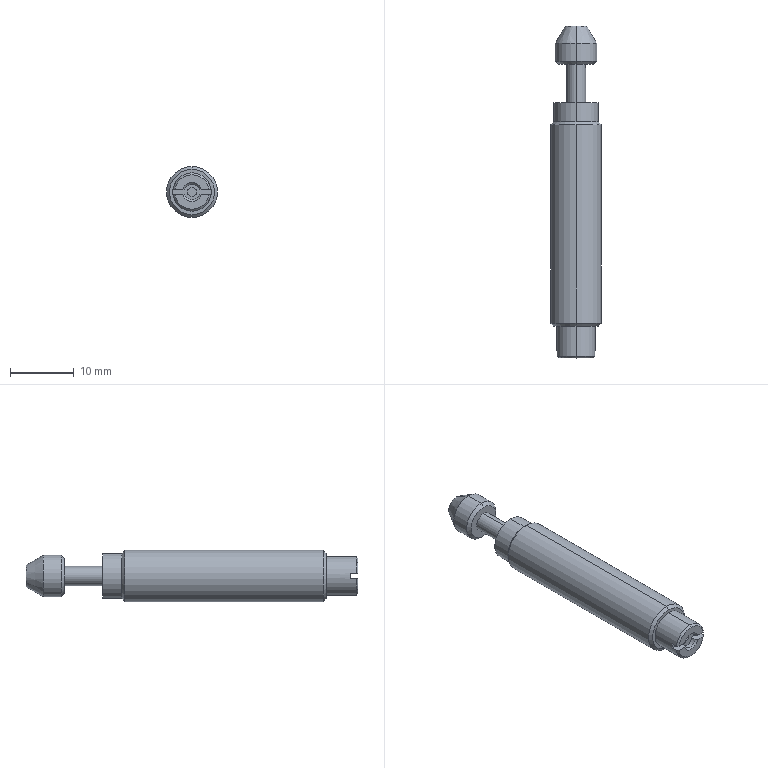Part | SolidWorks | features BaseBody 1 | 1 solid | 46 faces | box 8 x 52 x 8 mm | volume 2052 mm3 | plane 19 | cone 15 | cylinder 12 | commonest cylinder face diameters 2.459 x2 3 x2 6 x2 6.5 x2 7 x2 8 x2
STEP:
#1=CARTESIAN_POINT('',(0.,5.46,4.));
#2=VERTEX_POINT('',#1);
#3=CARTESIAN_POINT('',(0.,5.46,-4.));
#4=VERTEX_POINT('',#3);
#5=CARTESIAN_POINT('',(0.,5.46,0.));
#6=DIRECTION('',(0.,1.,0.));
#7=DIRECTION('',(0.,0.,1.));
#8=AXIS2_PLACEMENT_3D('',#5,#6,#7);
#9=CIRCLE('',#8,4.);
#10=EDGE_CURVE('',#2,#4,#9,.T.);
#11=ORIENTED_EDGE('',*,*,#10,.T.);
#12=CARTESIAN_POINT('',(0.,36.54,-4.));
#13=VERTEX_POINT('',#12);
#14=CARTESIAN_POINT('',(0.,0.,-4.));
#15=DIRECTION('',(0.,1.,0.));
#16=VECTOR('',#15,1000.);
#17=LINE('',#14,#16);
#18=EDGE_CURVE('',#4,#13,#17,.T.);
#19=ORIENTED_EDGE('',*,*,#18,.T.);
#20=CARTESIAN_POINT('',(0.,36.54,4.));
#21=VERTEX_POINT('',#20);
#22=CARTESIAN_POINT('',(0.,36.54,0.));
#23=DIRECTION('',(0.,-1.,0.));
#24=DIRECTION('',(0.,0.,1.));
#25=AXIS2_PLACEMENT_3D('',#22,#23,#24);
#26=CIRCLE('',#25,4.);
#27=EDGE_CURVE('',#13,#21,#26,.T.);
#28=ORIENTED_EDGE('',*,*,#27,.T.);
#29=CARTESIAN_POINT('',(0.,0.,4.));
#30=DIRECTION('',(0.,1.,0.));
#31=VECTOR('',#30,1000.);
#32=LINE('',#29,#31);
#33=EDGE_CURVE('',#2,#21,#32,.T.);
#34=ORIENTED_EDGE('',*,*,#33,.F.);
#35=EDGE_LOOP('',(#11,#19,#28,#34));
#36=FACE_OUTER_BOUND('',#35,.T.);
#37=CARTESIAN_POINT('',(0.,0.,0.));
#38=DIRECTION('',(0.,1.,0.));
#39=DIRECTION('',(0.,0.,1.));
#40=AXIS2_PLACEMENT_3D('',#37,#38,#39);
#41=CYLINDRICAL_SURFACE('',#40,4.);
#42=ADVANCED_FACE('',(#36),#41,.T.);
#43=CARTESIAN_POINT('',(0.,37.,-3.54));
#44=VERTEX_POINT('',#43);
#45=CARTESIAN_POINT('',(0.,37.,3.54));
#46=VERTEX_POINT('',#45);
#47=CARTESIAN_POINT('',(0.,37.,0.));
#48=DIRECTION('',(0.,-1.,0.));
#49=DIRECTION('',(0.,0.,-1.));
#50=AXIS2_PLACEMENT_3D('',#47,#48,#49);
#51=CIRCLE('',#50,3.54);
#52=EDGE_CURVE('',#44,#46,#51,.T.);
#53=ORIENTED_EDGE('',*,*,#52,.T.);
#54=CARTESIAN_POINT('',(0.,36.54,4.));
#55=DIRECTION('',(0.,-0.7071,0.7071));
#56=VECTOR('',#55,1000.);
#57=LINE('',#54,#56);
#58=EDGE_CURVE('',#46,#21,#57,.T.);
#59=ORIENTED_EDGE('',*,*,#58,.T.);
#60=ORIENTED_EDGE('',*,*,#27,.F.);
#61=CARTESIAN_POINT('',(0.,36.54,-4.));
#62=DIRECTION('',(0.,-0.7071,-0.7071));
#63=VECTOR('',#62,1000.);
#64=LINE('',#61,#63);
#65=EDGE_CURVE('',#44,#13,#64,.T.);
#66=ORIENTED_EDGE('',*,*,#65,.F.);
#67=EDGE_LOOP('',(#53,#59,#60,#66));
#68=FACE_OUTER_BOUND('',#67,.T.);
#69=CARTESIAN_POINT('',(0.,36.54,0.));
#70=DIRECTION('',(0.,-1.,0.));
#71=DIRECTION('',(0.,0.,-1.));
#72=AXIS2_PLACEMENT_3D('',#69,#70,#71);
#73=CONICAL_SURFACE('',#72,4.,0.7854);
#74=ADVANCED_FACE('',(#68),#73,.T.);
#75=CARTESIAN_POINT('',(0.,5.,3.54));
#76=VERTEX_POINT('',#75);
#77=CARTESIAN_POINT('',(0.,5.,-3.54));
#78=VERTEX_POINT('',#77);
#79=CARTESIAN_POINT('',(0.,5.,0.));
#80=DIRECTION('',(0.,1.,0.));
#81=DIRECTION('',(0.,0.,1.));
#82=AXIS2_PLACEMENT_3D('',#79,#80,#81);
#83=CIRCLE('',#82,3.54);
#84=EDGE_CURVE('',#76,#78,#83,.T.);
#85=ORIENTED_EDGE('',*,*,#84,.T.);
#86=CARTESIAN_POINT('',(0.,5.46,-4.));
#87=DIRECTION('',(0.,0.7071,-0.7071));
#88=VECTOR('',#87,1000.);
#89=LINE('',#86,#88);
#90=EDGE_CURVE('',#78,#4,#89,.T.);
#91=ORIENTED_EDGE('',*,*,#90,.T.);
#92=ORIENTED_EDGE('',*,*,#10,.F.);
#93=CARTESIAN_POINT('',(0.,5.46,4.));
#94=DIRECTION('',(0.,0.7071,0.7071));
#95=VECTOR('',#94,1000.);
#96=LINE('',#93,#95);
#97=EDGE_CURVE('',#76,#2,#96,.T.);
#98=ORIENTED_EDGE('',*,*,#97,.F.);
#99=EDGE_LOOP('',(#85,#91,#92,#98));
#100=FACE_OUTER_BOUND('',#99,.T.);
#101=CARTESIAN_POINT('',(0.,5.46,0.));
#102=DIRECTION('',(0.,1.,0.));
#103=DIRECTION('',(0.,0.,1.));
#104=AXIS2_PLACEMENT_3D('',#101,#102,#103);
#105=CONICAL_SURFACE('',#104,4.,0.7854);
#106=ADVANCED_FACE('',(#100),#105,.T.);
#107=CARTESIAN_POINT('',(0.,37.,3.5));
#108=VERTEX_POINT('',#107);
#109=CARTESIAN_POINT('',(0.,37.,-3.5));
#110=VERTEX_POINT('',#109);
#111=CARTESIAN_POINT('',(0.,37.,0.));
#112=DIRECTION('',(0.,1.,0.));
#113=DIRECTION('',(0.,0.,1.));
#114=AXIS2_PLACEMENT_3D('',#111,#112,#113);
#115=CIRCLE('',#114,3.5);
#116=EDGE_CURVE('',#108,#110,#115,.T.);
#117=ORIENTED_EDGE('',*,*,#116,.T.);
#118=CARTESIAN_POINT('',(0.,40.,-3.5));
#119=VERTEX_POINT('',#118);
#120=CARTESIAN_POINT('',(0.,0.,-3.5));
#121=DIRECTION('',(0.,1.,0.));
#122=VECTOR('',#121,1000.);
#123=LINE('',#120,#122);
#124=EDGE_CURVE('',#110,#119,#123,.T.);
#125=ORIENTED_EDGE('',*,*,#124,.T.);
#126=CARTESIAN_POINT('',(0.,40.,3.5));
#127=VERTEX_POINT('',#126);
#128=CARTESIAN_POINT('',(0.,40.,0.));
#129=DIRECTION('',(0.,-1.,0.));
#130=DIRECTION('',(0.,0.,1.));
#131=AXIS2_PLACEMENT_3D('',#128,#129,#130);
#132=CIRCLE('',#131,3.5);
#133=EDGE_CURVE('',#119,#127,#132,.T.);
#134=ORIENTED_EDGE('',*,*,#133,.T.);
#135=CARTESIAN_POINT('',(0.,0.,3.5));
#136=DIRECTION('',(0.,1.,0.));
#137=VECTOR('',#136,1000.);
#138=LINE('',#135,#137);
#139=EDGE_CURVE('',#108,#127,#138,.T.);
#140=ORIENTED_EDGE('',*,*,#139,.F.);
#141=EDGE_LOOP('',(#117,#125,#134,#140));
#142=FACE_OUTER_BOUND('',#141,.T.);
#143=CARTESIAN_POINT('',(0.,0.,0.));
#144=DIRECTION('',(0.,1.,0.));
#145=DIRECTION('',(0.,0.,1.));
#146=AXIS2_PLACEMENT_3D('',#143,#144,#145);
#147=CYLINDRICAL_SURFACE('',#146,3.5);
#148=ADVANCED_FACE('',(#142),#147,.T.);
#149=CARTESIAN_POINT('',(2.973,0.3,-0.4));
#150=VERTEX_POINT('',#149);
#151=CARTESIAN_POINT('',(0.,0.3,-3.));
#152=VERTEX_POINT('',#151);
#153=CARTESIAN_POINT('',(0.,0.3,0.));
#154=DIRECTION('',(0.,1.,0.));
#155=DIRECTION('',(0.,0.,1.));
#156=AXIS2_PLACEMENT_3D('',#153,#154,#155);
#157=CIRCLE('',#156,3.);
#158=EDGE_CURVE('',#150,#152,#157,.T.);
#159=ORIENTED_EDGE('',*,*,#158,.T.);
#160=CARTESIAN_POINT('',(0.,5.,-3.));
#161=VERTEX_POINT('',#160);
#162=CARTESIAN_POINT('',(0.,0.,-3.));
#163=DIRECTION('',(0.,1.,0.));
#164=VECTOR('',#163,1000.);
#165=LINE('',#162,#164);
#166=EDGE_CURVE('',#152,#161,#165,.T.);
#167=ORIENTED_EDGE('',*,*,#166,.T.);
#168=CARTESIAN_POINT('',(0.,5.,3.));
#169=VERTEX_POINT('',#168);
#170=CARTESIAN_POINT('',(0.,5.,0.));
#171=DIRECTION('',(0.,-1.,0.));
#172=DIRECTION('',(0.,0.,1.));
#173=AXIS2_PLACEMENT_3D('',#170,#171,#172);
#174=CIRCLE('',#173,3.);
#175=EDGE_CURVE('',#161,#169,#174,.T.);
#176=ORIENTED_EDGE('',*,*,#175,.T.);
#177=CARTESIAN_POINT('',(0.,0.3,3.));
#178=VERTEX_POINT('',#177);
#179=CARTESIAN_POINT('',(0.,0.,3.));
#180=DIRECTION('',(0.,1.,0.));
#181=VECTOR('',#180,1000.);
#182=LINE('',#179,#181);
#183=EDGE_CURVE('',#178,#169,#182,.T.);
#184=ORIENTED_EDGE('',*,*,#183,.F.);
#185=CARTESIAN_POINT('',(2.973,0.3,0.4));
#186=VERTEX_POINT('',#185);
#187=CARTESIAN_POINT('',(0.,0.3,0.));
#188=DIRECTION('',(0.,1.,0.));
#189=DIRECTION('',(0.,0.,1.));
#190=AXIS2_PLACEMENT_3D('',#187,#188,#189);
#191=CIRCLE('',#190,3.);
#192=EDGE_CURVE('',#178,#186,#191,.T.);
#193=ORIENTED_EDGE('',*,*,#192,.T.);
#194=CARTESIAN_POINT('',(2.973,1.2,0.4));
#195=VERTEX_POINT('',#194);
#196=CARTESIAN_POINT('',(2.973,0.,0.4));
#197=DIRECTION('',(0.,1.,0.));
#198=VECTOR('',#197,1000.);
#199=LINE('',#196,#198);
#200=EDGE_CURVE('',#186,#195,#199,.T.);
#201=ORIENTED_EDGE('',*,*,#200,.T.);
#202=CARTESIAN_POINT('',(2.973,1.2,-0.4));
#203=VERTEX_POINT('',#202);
#204=CARTESIAN_POINT('',(0.,1.2,0.));
#205=DIRECTION('',(0.,-1.,0.));
#206=DIRECTION('',(0.,0.,1.));
#207=AXIS2_PLACEMENT_3D('',#204,#205,#206);
#208=CIRCLE('',#207,3.);
#209=EDGE_CURVE('',#203,#195,#208,.T.);
#210=ORIENTED_EDGE('',*,*,#209,.F.);
#211=CARTESIAN_POINT('',(2.973,0.,-0.4));
#212=DIRECTION('',(0.,-1.,0.));
#213=VECTOR('',#212,1000.);
#214=LINE('',#211,#213);
#215=EDGE_CURVE('',#203,#150,#214,.T.);
#216=ORIENTED_EDGE('',*,*,#215,.T.);
#217=EDGE_LOOP('',(#159,#167,#176,#184,#193,#201,#210,#216));
#218=FACE_OUTER_BOUND('',#217,.T.);
#219=CARTESIAN_POINT('',(0.,0.,0.));
#220=DIRECTION('',(0.,1.,0.));
#221=DIRECTION('',(0.,0.,1.));
#222=AXIS2_PLACEMENT_3D('',#219,#220,#221);
#223=CYLINDRICAL_SURFACE('',#222,3.);
#224=ADVANCED_FACE('',(#218),#223,.T.);
#225=CARTESIAN_POINT('',(-2.67,0.,0.4));
#226=VERTEX_POINT('',#225);
#227=CARTESIAN_POINT('',(0.,0.,2.7));
#228=VERTEX_POINT('',#227);
#229=CARTESIAN_POINT('',(0.,0.,0.));
#230=DIRECTION('',(0.,1.,0.));
#231=DIRECTION('',(0.,0.,1.));
#232=AXIS2_PLACEMENT_3D('',#229,#230,#231);
#233=CIRCLE('',#232,2.7);
#234=EDGE_CURVE('',#226,#228,#233,.T.);
#235=ORIENTED_EDGE('',*,*,#234,.T.);
#236=CARTESIAN_POINT('',(0.,0.3,3.));
#237=DIRECTION('',(0.,0.7071,0.7071));
#238=VECTOR('',#237,1000.);
#239=LINE('',#236,#238);
#240=EDGE_CURVE('',#228,#178,#239,.T.);
#241=ORIENTED_EDGE('',*,*,#240,.T.);
#242=CARTESIAN_POINT('',(-2.973,0.3,0.4));
#243=VERTEX_POINT('',#242);
#244=CARTESIAN_POINT('',(0.,0.3,0.));
#245=DIRECTION('',(0.,1.,0.));
#246=DIRECTION('',(0.,0.,1.));
#247=AXIS2_PLACEMENT_3D('',#244,#245,#246);
#248=CIRCLE('',#247,3.);
#249=EDGE_CURVE('',#243,#178,#248,.T.);
#250=ORIENTED_EDGE('',*,*,#249,.F.);
#251=CARTESIAN_POINT('',(-2.973,0.3,0.4));
#252=CARTESIAN_POINT('',(-2.872,0.1999,0.4));
#253=CARTESIAN_POINT('',(-2.771,0.09994,0.4));
#254=CARTESIAN_POINT('',(-2.67,0.,0.4));
#255=B_SPLINE_CURVE_WITH_KNOTS('',3,(#251,#252,#253,#254),.UNSPECIFIED.,.F.,.F.,(4,4),(0.,0.0004264),.UNSPECIFIED.);
#256=EDGE_CURVE('',#243,#226,#255,.T.);
#257=ORIENTED_EDGE('',*,*,#256,.T.);
#258=EDGE_LOOP('',(#235,#241,#250,#257));
#259=FACE_OUTER_BOUND('',#258,.T.);
#260=CARTESIAN_POINT('',(0.,0.3,0.));
#261=DIRECTION('',(0.,1.,0.));
#262=DIRECTION('',(0.,0.,1.));
#263=AXIS2_PLACEMENT_3D('',#260,#261,#262);
#264=CONICAL_SURFACE('',#263,3.,0.7854);
#265=ADVANCED_FACE('',(#259),#264,.T.);
#266=CARTESIAN_POINT('',(0.,40.,1.5));
#267=VERTEX_POINT('',#266);
#268=CARTESIAN_POINT('',(0.,40.,-1.5));
#269=VERTEX_POINT('',#268);
#270=CARTESIAN_POINT('',(0.,40.,0.));
#271=DIRECTION('',(0.,1.,0.));
#272=DIRECTION('',(0.,0.,1.));
#273=AXIS2_PLACEMENT_3D('',#270,#271,#272);
#274=CIRCLE('',#273,1.5);
#275=EDGE_CURVE('',#267,#269,#274,.T.);
#276=ORIENTED_EDGE('',*,*,#275,.T.);
#277=CARTESIAN_POINT('',(0.,46.,-1.5));
#278=VERTEX_POINT('',#277);
#279=CARTESIAN_POINT('',(0.,0.,-1.5));
#280=DIRECTION('',(0.,1.,0.));
#281=VECTOR('',#280,1000.);
#282=LINE('',#279,#281);
#283=EDGE_CURVE('',#269,#278,#282,.T.);
#284=ORIENTED_EDGE('',*,*,#283,.T.);
#285=CARTESIAN_POINT('',(0.,46.,1.5));
#286=VERTEX_POINT('',#285);
#287=CARTESIAN_POINT('',(0.,46.,0.));
#288=DIRECTION('',(0.,-1.,0.));
#289=DIRECTION('',(0.,0.,1.));
#290=AXIS2_PLACEMENT_3D('',#287,#288,#289);
#291=CIRCLE('',#290,1.5);
#292=EDGE_CURVE('',#278,#286,#291,.T.);
#293=ORIENTED_EDGE('',*,*,#292,.T.);
#294=CARTESIAN_POINT('',(0.,0.,1.5));
#295=DIRECTION('',(0.,1.,0.));
#296=VECTOR('',#295,1000.);
#297=LINE('',#294,#296);
#298=EDGE_CURVE('',#267,#286,#297,.T.);
#299=ORIENTED_EDGE('',*,*,#298,.F.);
#300=EDGE_LOOP('',(#276,#284,#293,#299));
#301=FACE_OUTER_BOUND('',#300,.T.);
#302=CARTESIAN_POINT('',(0.,0.,0.));
#303=DIRECTION('',(0.,1.,0.));
#304=DIRECTION('',(0.,0.,1.));
#305=AXIS2_PLACEMENT_3D('',#302,#303,#304);
#306=CYLINDRICAL_SURFACE('',#305,1.5);
#307=ADVANCED_FACE('',(#301),#306,.T.);
#308=CARTESIAN_POINT('',(0.,46.,2.75));
#309=VERTEX_POINT('',#308);
#310=CARTESIAN_POINT('',(0.,46.,-2.75));
#311=VERTEX_POINT('',#310);
#312=CARTESIAN_POINT('',(0.,46.,0.));
#313=DIRECTION('',(0.,1.,0.));
#314=DIRECTION('',(0.,0.,1.));
#315=AXIS2_PLACEMENT_3D('',#312,#313,#314);
#316=CIRCLE('',#315,2.75);
#317=EDGE_CURVE('',#309,#311,#316,.T.);
#318=ORIENTED_EDGE('',*,*,#317,.T.);
#319=CARTESIAN_POINT('',(0.,46.5,-3.25));
#320=VERTEX_POINT('',#319);
#321=CARTESIAN_POINT('',(0.,46.5,-3.25));
#322=DIRECTION('',(0.,0.7071,-0.7071));
#323=VECTOR('',#322,1000.);
#324=LINE('',#321,#323);
#325=EDGE_CURVE('',#311,#320,#324,.T.);
#326=ORIENTED_EDGE('',*,*,#325,.T.);
#327=CARTESIAN_POINT('',(0.,46.5,3.25));
#328=VERTEX_POINT('',#327);
#329=CARTESIAN_POINT('',(0.,46.5,0.));
#330=DIRECTION('',(0.,-1.,0.));
#331=DIRECTION('',(0.,0.,1.));
#332=AXIS2_PLACEMENT_3D('',#329,#330,#331);
#333=CIRCLE('',#332,3.25);
#334=EDGE_CURVE('',#320,#328,#333,.T.);
#335=ORIENTED_EDGE('',*,*,#334,.T.);
#336=CARTESIAN_POINT('',(0.,46.5,3.25));
#337=DIRECTION('',(0.,0.7071,0.7071));
#338=VECTOR('',#337,1000.);
#339=LINE('',#336,#338);
#340=EDGE_CURVE('',#309,#328,#339,.T.);
#341=ORIENTED_EDGE('',*,*,#340,.F.);
#342=EDGE_LOOP('',(#318,#326,#335,#341));
#343=FACE_OUTER_BOUND('',#342,.T.);
#344=CARTESIAN_POINT('',(0.,46.5,0.));
#345=DIRECTION('',(0.,1.,0.));
#346=DIRECTION('',(0.,0.,1.));
#347=AXIS2_PLACEMENT_3D('',#344,#345,#346);
#348=CONICAL_SURFACE('',#347,3.25,0.7854);
#349=ADVANCED_FACE('',(#343),#348,.T.);
#350=ORIENTED_EDGE('',*,*,#334,.F.);
#351=CARTESIAN_POINT('',(0.,49.333,-3.25));
#352=VERTEX_POINT('',#351);
#353=CARTESIAN_POINT('',(0.,0.,-3.25));
#354=DIRECTION('',(0.,1.,0.));
#355=VECTOR('',#354,1000.);
#356=LINE('',#353,#355);
#357=EDGE_CURVE('',#320,#352,#356,.T.);
#358=ORIENTED_EDGE('',*,*,#357,.T.);
#359=CARTESIAN_POINT('',(0.,49.333,3.25));
#360=VERTEX_POINT('',#359);
#361=CARTESIAN_POINT('',(0.,49.333,0.));
#362=DIRECTION('',(0.,-1.,0.));
#363=DIRECTION('',(0.,0.,1.));
#364=AXIS2_PLACEMENT_3D('',#361,#362,#363);
#365=CIRCLE('',#364,3.25);
#366=EDGE_CURVE('',#352,#360,#365,.T.);
#367=ORIENTED_EDGE('',*,*,#366,.T.);
#368=CARTESIAN_POINT('',(0.,0.,3.25));
#369=DIRECTION('',(0.,1.,0.));
#370=VECTOR('',#369,1000.);
#371=LINE('',#368,#370);
#372=EDGE_CURVE('',#328,#360,#371,.T.);
#373=ORIENTED_EDGE('',*,*,#372,.F.);
#374=EDGE_LOOP('',(#350,#358,#367,#373));
#375=FACE_OUTER_BOUND('',#374,.T.);
#376=CARTESIAN_POINT('',(0.,0.,0.));
#377=DIRECTION('',(0.,1.,0.));
#378=DIRECTION('',(0.,0.,1.));
#379=AXIS2_PLACEMENT_3D('',#376,#377,#378);
#380=CYLINDRICAL_SURFACE('',#379,3.25);
#381=ADVANCED_FACE('',(#375),#380,.T.);
#382=CARTESIAN_POINT('',(0.,52.,-1.71));
#383=VERTEX_POINT('',#382);
#384=CARTESIAN_POINT('',(0.,52.,1.71));
#385=VERTEX_POINT('',#384);
#386=CARTESIAN_POINT('',(0.,52.,0.));
#387=DIRECTION('',(0.,-1.,0.));
#388=DIRECTION('',(0.,0.,-1.));
#389=AXIS2_PLACEMENT_3D('',#386,#387,#388);
#390=CIRCLE('',#389,1.71);
#391=EDGE_CURVE('',#383,#385,#390,.T.);
#392=ORIENTED_EDGE('',*,*,#391,.T.);
#393=CARTESIAN_POINT('',(0.,49.333,3.25));
#394=DIRECTION('',(0.,-0.866,0.5));
#395=VECTOR('',#394,1000.);
#396=LINE('',#393,#395);
#397=EDGE_CURVE('',#385,#360,#396,.T.);
#398=ORIENTED_EDGE('',*,*,#397,.T.);
#399=ORIENTED_EDGE('',*,*,#366,.F.);
#400=CARTESIAN_POINT('',(0.,49.333,-3.25));
#401=DIRECTION('',(0.,-0.866,-0.5));
#402=VECTOR('',#401,1000.);
#403=LINE('',#400,#402);
#404=EDGE_CURVE('',#383,#352,#403,.T.);
#405=ORIENTED_EDGE('',*,*,#404,.F.);
#406=EDGE_LOOP('',(#392,#398,#399,#405));
#407=FACE_OUTER_BOUND('',#406,.T.);
#408=CARTESIAN_POINT('',(0.,49.333,0.));
#409=DIRECTION('',(0.,-1.,0.));
#410=DIRECTION('',(0.,0.,-1.));
#411=AXIS2_PLACEMENT_3D('',#408,#409,#410);
#412=CONICAL_SURFACE('',#411,3.25,0.5236);
#413=ADVANCED_FACE('',(#407),#412,.T.);
#414=ORIENTED_EDGE('',*,*,#18,.F.);
#415=CARTESIAN_POINT('',(0.,5.46,0.));
#416=DIRECTION('',(0.,1.,0.));
#417=DIRECTION('',(0.,0.,1.));
#418=AXIS2_PLACEMENT_3D('',#415,#416,#417);
#419=CIRCLE('',#418,4.);
#420=EDGE_CURVE('',#4,#2,#419,.T.);
#421=ORIENTED_EDGE('',*,*,#420,.T.);
#422=ORIENTED_EDGE('',*,*,#33,.T.);
#423=CARTESIAN_POINT('',(0.,36.54,0.));
#424=DIRECTION('',(0.,-1.,0.));
#425=DIRECTION('',(0.,0.,1.));
#426=AXIS2_PLACEMENT_3D('',#423,#424,#425);
#427=CIRCLE('',#426,4.);
#428=EDGE_CURVE('',#21,#13,#427,.T.);
#429=ORIENTED_EDGE('',*,*,#428,.T.);
#430=EDGE_LOOP('',(#414,#421,#422,#429));
#431=FACE_OUTER_BOUND('',#430,.T.);
#432=CARTESIAN_POINT('',(0.,0.,0.));
#433=DIRECTION('',(0.,1.,0.));
#434=DIRECTION('',(0.,0.,1.));
#435=AXIS2_PLACEMENT_3D('',#432,#433,#434);
#436=CYLINDRICAL_SURFACE('',#435,4.);
#437=ADVANCED_FACE('',(#431),#436,.T.);
#438=ORIENTED_EDGE('',*,*,#58,.F.);
#439=CARTESIAN_POINT('',(0.,37.,0.));
#440=DIRECTION('',(0.,-1.,0.));
#441=DIRECTION('',(0.,0.,-1.));
#442=AXIS2_PLACEMENT_3D('',#439,#440,#441);
#443=CIRCLE('',#442,3.54);
#444=EDGE_CURVE('',#46,#44,#443,.T.);
#445=ORIENTED_EDGE('',*,*,#444,.T.);
#446=ORIENTED_EDGE('',*,*,#65,.T.);
#447=ORIENTED_EDGE('',*,*,#428,.F.);
#448=EDGE_LOOP('',(#438,#445,#446,#447));
#449=FACE_OUTER_BOUND('',#448,.T.);
#450=CARTESIAN_POINT('',(0.,36.54,0.));
#451=DIRECTION('',(0.,-1.,0.));
#452=DIRECTION('',(0.,0.,-1.));
#453=AXIS2_PLACEMENT_3D('',#450,#451,#452);
#454=CONICAL_SURFACE('',#453,4.,0.7854);
#455=ADVANCED_FACE('',(#449),#454,.T.);
#456=ORIENTED_EDGE('',*,*,#90,.F.);
#457=CARTESIAN_POINT('',(0.,5.,0.));
#458=DIRECTION('',(0.,1.,0.));
#459=DIRECTION('',(0.,0.,1.));
#460=AXIS2_PLACEMENT_3D('',#457,#458,#459);
#461=CIRCLE('',#460,3.54);
#462=EDGE_CURVE('',#78,#76,#461,.T.);
#463=ORIENTED_EDGE('',*,*,#462,.T.);
#464=ORIENTED_EDGE('',*,*,#97,.T.);
#465=ORIENTED_EDGE('',*,*,#420,.F.);
#466=EDGE_LOOP('',(#456,#463,#464,#465));
#467=FACE_OUTER_BOUND('',#466,.T.);
#468=CARTESIAN_POINT('',(0.,5.46,0.));
#469=DIRECTION('',(0.,1.,0.));
#470=DIRECTION('',(0.,0.,1.));
#471=AXIS2_PLACEMENT_3D('',#468,#469,#470);
#472=CONICAL_SURFACE('',#471,4.,0.7854);
#473=ADVANCED_FACE('',(#467),#472,.T.);
#474=ORIENTED_EDGE('',*,*,#116,.F.);
#475=CARTESIAN_POINT('',(0.,37.,0.));
#476=DIRECTION('',(0.,1.,0.));
#477=DIRECTION('',(0.,0.,1.));
#478=AXIS2_PLACEMENT_3D('',#475,#476,#477);
#479=CIRCLE('',#478,3.5);
#480=EDGE_CURVE('',#110,#108,#479,.T.);
#481=ORIENTED_EDGE('',*,*,#480,.F.);
#482=EDGE_LOOP('',(#474,#481));
#483=FACE_BOUND('',#482,.T.);
#484=ORIENTED_EDGE('',*,*,#52,.F.);
#485=ORIENTED_EDGE('',*,*,#444,.F.);
#486=EDGE_LOOP('',(#484,#485));
#487=FACE_OUTER_BOUND('',#486,.T.);
#488=CARTESIAN_POINT('',(3.5,37.,0.));
#489=DIRECTION('',(0.,-1.,0.));
#490=DIRECTION('',(0.,0.,-1.));
#491=AXIS2_PLACEMENT_3D('',#488,#489,#490);
#492=PLANE('',#491);
#493=ADVANCED_FACE('',(#483,#487),#492,.F.);
#494=ORIENTED_EDGE('',*,*,#84,.F.);
#495=ORIENTED_EDGE('',*,*,#462,.F.);
#496=EDGE_LOOP('',(#494,#495));
#497=FACE_OUTER_BOUND('',#496,.T.);
#498=CARTESIAN_POINT('',(0.,5.,0.));
#499=DIRECTION('',(0.,-1.,0.));
#500=DIRECTION('',(0.,0.,1.));
#501=AXIS2_PLACEMENT_3D('',#498,#499,#500);
#502=CIRCLE('',#501,3.);
#503=EDGE_CURVE('',#169,#161,#502,.T.);
#504=ORIENTED_EDGE('',*,*,#503,.F.);
#505=ORIENTED_EDGE('',*,*,#175,.F.);
#506=EDGE_LOOP('',(#504,#505));
#507=FACE_BOUND('',#506,.T.);
#508=CARTESIAN_POINT('',(3.54,5.,0.));
#509=DIRECTION('',(0.,1.,0.));
#510=DIRECTION('',(0.,0.,1.));
#511=AXIS2_PLACEMENT_3D('',#508,#509,#510);
#512=PLANE('',#511);
#513=ADVANCED_FACE('',(#497,#507),#512,.F.);
#514=ORIENTED_EDGE('',*,*,#124,.F.);
#515=ORIENTED_EDGE('',*,*,#480,.T.);
#516=ORIENTED_EDGE('',*,*,#139,.T.);
#517=CARTESIAN_POINT('',(0.,40.,0.));
#518=DIRECTION('',(0.,-1.,0.));
#519=DIRECTION('',(0.,0.,1.));
#520=AXIS2_PLACEMENT_3D('',#517,#518,#519);
#521=CIRCLE('',#520,3.5);
#522=EDGE_CURVE('',#127,#119,#521,.T.);
#523=ORIENTED_EDGE('',*,*,#522,.T.);
#524=EDGE_LOOP('',(#514,#515,#516,#523));
#525=FACE_OUTER_BOUND('',#524,.T.);
#526=CARTESIAN_POINT('',(0.,0.,0.));
#527=DIRECTION('',(0.,1.,0.));
#528=DIRECTION('',(0.,0.,1.));
#529=AXIS2_PLACEMENT_3D('',#526,#527,#528);
#530=CYLINDRICAL_SURFACE('',#529,3.5);
#531=ADVANCED_FACE('',(#525),#530,.T.);
#532=ORIENTED_EDGE('',*,*,#166,.F.);
#533=CARTESIAN_POINT('',(-2.973,0.3,-0.4));
#534=VERTEX_POINT('',#533);
#535=CARTESIAN_POINT('',(0.,0.3,0.));
#536=DIRECTION('',(0.,1.,0.));
#537=DIRECTION('',(0.,0.,1.));
#538=AXIS2_PLACEMENT_3D('',#535,#536,#537);
#539=CIRCLE('',#538,3.);
#540=EDGE_CURVE('',#152,#534,#539,.T.);
#541=ORIENTED_EDGE('',*,*,#540,.T.);
#542=CARTESIAN_POINT('',(-2.973,1.2,-0.4));
#543=VERTEX_POINT('',#542);
#544=CARTESIAN_POINT('',(-2.973,0.,-0.4));
#545=DIRECTION('',(0.,1.,0.));
#546=VECTOR('',#545,1000.);
#547=LINE('',#544,#546);
#548=EDGE_CURVE('',#534,#543,#547,.T.);
#549=ORIENTED_EDGE('',*,*,#548,.T.);
#550=CARTESIAN_POINT('',(-2.973,1.2,0.4));
#551=VERTEX_POINT('',#550);
#552=CARTESIAN_POINT('',(0.,1.2,0.));
#553=DIRECTION('',(0.,-1.,0.));
#554=DIRECTION('',(0.,0.,1.));
#555=AXIS2_PLACEMENT_3D('',#552,#553,#554);
#556=CIRCLE('',#555,3.);
#557=EDGE_CURVE('',#551,#543,#556,.T.);
#558=ORIENTED_EDGE('',*,*,#557,.F.);
#559=CARTESIAN_POINT('',(-2.973,0.,0.4));
#560=DIRECTION('',(0.,-1.,0.));
#561=VECTOR('',#560,1000.);
#562=LINE('',#559,#561);
#563=EDGE_CURVE('',#551,#243,#562,.T.);
#564=ORIENTED_EDGE('',*,*,#563,.T.);
#565=ORIENTED_EDGE('',*,*,#249,.T.);
#566=ORIENTED_EDGE('',*,*,#183,.T.);
#567=ORIENTED_EDGE('',*,*,#503,.T.);
#568=EDGE_LOOP('',(#532,#541,#549,#558,#564,#565,#566,#567));
#569=FACE_OUTER_BOUND('',#568,.T.);
#570=CARTESIAN_POINT('',(0.,0.,0.));
#571=DIRECTION('',(0.,1.,0.));
#572=DIRECTION('',(0.,0.,1.));
#573=AXIS2_PLACEMENT_3D('',#570,#571,#572);
#574=CYLINDRICAL_SURFACE('',#573,3.);
#575=ADVANCED_FACE('',(#569),#574,.T.);
#576=ORIENTED_EDGE('',*,*,#275,.F.);
#577=CARTESIAN_POINT('',(0.,40.,0.));
#578=DIRECTION('',(0.,1.,0.));
#579=DIRECTION('',(0.,0.,1.));
#580=AXIS2_PLACEMENT_3D('',#577,#578,#579);
#581=CIRCLE('',#580,1.5);
#582=EDGE_CURVE('',#269,#267,#581,.T.);
#583=ORIENTED_EDGE('',*,*,#582,.F.);
#584=EDGE_LOOP('',(#576,#583));
#585=FACE_BOUND('',#584,.T.);
#586=ORIENTED_EDGE('',*,*,#522,.F.);
#587=ORIENTED_EDGE('',*,*,#133,.F.);
#588=EDGE_LOOP('',(#586,#587));
#589=FACE_OUTER_BOUND('',#588,.T.);
#590=CARTESIAN_POINT('',(1.5,40.,0.));
#591=DIRECTION('',(0.,-1.,0.));
#592=DIRECTION('',(0.,0.,-1.));
#593=AXIS2_PLACEMENT_3D('',#590,#591,#592);
#594=PLANE('',#593);
#595=ADVANCED_FACE('',(#585,#589),#594,.F.);
#596=ORIENTED_EDGE('',*,*,#240,.F.);
#597=CARTESIAN_POINT('',(2.67,0.,0.4));
#598=VERTEX_POINT('',#597);
#599=CARTESIAN_POINT('',(0.,0.,0.));
#600=DIRECTION('',(0.,1.,0.));
#601=DIRECTION('',(0.,0.,1.));
#602=AXIS2_PLACEMENT_3D('',#599,#600,#601);
#603=CIRCLE('',#602,2.7);
#604=EDGE_CURVE('',#228,#598,#603,.T.);
#605=ORIENTED_EDGE('',*,*,#604,.T.);
#606=CARTESIAN_POINT('',(2.67,0.,0.4));
#607=CARTESIAN_POINT('',(2.771,0.09994,0.4));
#608=CARTESIAN_POINT('',(2.872,0.1999,0.4));
#609=CARTESIAN_POINT('',(2.973,0.3,0.4));
#610=B_SPLINE_CURVE_WITH_KNOTS('',3,(#606,#607,#608,#609),.UNSPECIFIED.,.F.,.F.,(4,4),(0.,0.0004264),.UNSPECIFIED.);
#611=EDGE_CURVE('',#598,#186,#610,.T.);
#612=ORIENTED_EDGE('',*,*,#611,.T.);
#613=ORIENTED_EDGE('',*,*,#192,.F.);
#614=EDGE_LOOP('',(#596,#605,#612,#613));
#615=FACE_OUTER_BOUND('',#614,.T.);
#616=CARTESIAN_POINT('',(0.,0.3,0.));
#617=DIRECTION('',(0.,1.,0.));
#618=DIRECTION('',(0.,0.,1.));
#619=AXIS2_PLACEMENT_3D('',#616,#617,#618);
#620=CONICAL_SURFACE('',#619,3.,0.7854);
#621=ADVANCED_FACE('',(#615),#620,.T.);
#622=CARTESIAN_POINT('',(-1.446,1.2,0.4));
#623=VERTEX_POINT('',#622);
#624=CARTESIAN_POINT('',(-1.163,0.9295,0.4));
#625=VERTEX_POINT('',#624);
#626=CARTESIAN_POINT('',(-1.446,1.2,0.4));
#627=CARTESIAN_POINT('',(-1.352,1.109,0.4));
#628=CARTESIAN_POINT('',(-1.257,1.019,0.4));
#629=CARTESIAN_POINT('',(-1.163,0.9295,0.4));
#630=B_SPLINE_CURVE_WITH_KNOTS('',3,(#626,#627,#628,#629),.UNSPECIFIED.,.F.,.F.,(4,4),(0.,0.0003915),.UNSPECIFIED.);
#631=EDGE_CURVE('',#623,#625,#630,.T.);
#632=ORIENTED_EDGE('',*,*,#631,.T.);
#633=CARTESIAN_POINT('',(-1.163,0.2705,0.4));
#634=VERTEX_POINT('',#633);
#635=CARTESIAN_POINT('',(-1.163,0.,0.4));
#636=DIRECTION('',(0.,-1.,0.));
#637=VECTOR('',#636,1000.);
#638=LINE('',#635,#637);
#639=EDGE_CURVE('',#625,#634,#638,.T.);
#640=ORIENTED_EDGE('',*,*,#639,.T.);
#641=CARTESIAN_POINT('',(-1.446,0.,0.4));
#642=VERTEX_POINT('',#641);
#643=CARTESIAN_POINT('',(-1.163,0.2705,0.4));
#644=CARTESIAN_POINT('',(-1.257,0.1808,0.4));
#645=CARTESIAN_POINT('',(-1.352,0.09057,0.4));
#646=CARTESIAN_POINT('',(-1.446,0.,0.4));
#647=B_SPLINE_CURVE_WITH_KNOTS('',3,(#643,#644,#645,#646),.UNSPECIFIED.,.F.,.F.,(4,4),(0.,0.0003915),.UNSPECIFIED.);
#648=EDGE_CURVE('',#634,#642,#647,.T.);
#649=ORIENTED_EDGE('',*,*,#648,.T.);
#650=CARTESIAN_POINT('',(0.,0.,0.4));
#651=DIRECTION('',(1.,0.,0.));
#652=VECTOR('',#651,1000.);
#653=LINE('',#650,#652);
#654=EDGE_CURVE('',#226,#642,#653,.T.);
#655=ORIENTED_EDGE('',*,*,#654,.F.);
#656=ORIENTED_EDGE('',*,*,#256,.F.);
#657=ORIENTED_EDGE('',*,*,#563,.F.);
#658=CARTESIAN_POINT('',(0.,1.2,0.4));
#659=DIRECTION('',(-1.,0.,0.));
#660=VECTOR('',#659,1000.);
#661=LINE('',#658,#660);
#662=EDGE_CURVE('',#623,#551,#661,.T.);
#663=ORIENTED_EDGE('',*,*,#662,.F.);
#664=EDGE_LOOP('',(#632,#640,#649,#655,#656,#657,#663));
#665=FACE_OUTER_BOUND('',#664,.T.);
#666=CARTESIAN_POINT('',(0.,0.,0.4));
#667=DIRECTION('',(0.,0.,1.));
#668=DIRECTION('',(1.,0.,0.));
#669=AXIS2_PLACEMENT_3D('',#666,#667,#668);
#670=PLANE('',#669);
#671=ADVANCED_FACE('',(#665),#670,.F.);
#672=CARTESIAN_POINT('',(-1.163,0.9295,-0.4));
#673=VERTEX_POINT('',#672);
#674=CARTESIAN_POINT('',(-1.446,1.2,-0.4));
#675=VERTEX_POINT('',#674);
#676=CARTESIAN_POINT('',(-1.163,0.9295,-0.4));
#677=CARTESIAN_POINT('',(-1.257,1.019,-0.4));
#678=CARTESIAN_POINT('',(-1.352,1.109,-0.4));
#679=CARTESIAN_POINT('',(-1.446,1.2,-0.4));
#680=B_SPLINE_CURVE_WITH_KNOTS('',3,(#676,#677,#678,#679),.UNSPECIFIED.,.F.,.F.,(4,4),(0.,0.0003915),.UNSPECIFIED.);
#681=EDGE_CURVE('',#673,#675,#680,.T.);
#682=ORIENTED_EDGE('',*,*,#681,.T.);
#683=CARTESIAN_POINT('',(0.,1.2,-0.4));
#684=DIRECTION('',(1.,0.,0.));
#685=VECTOR('',#684,1000.);
#686=LINE('',#683,#685);
#687=EDGE_CURVE('',#543,#675,#686,.T.);
#688=ORIENTED_EDGE('',*,*,#687,.F.);
#689=ORIENTED_EDGE('',*,*,#548,.F.);
#690=CARTESIAN_POINT('',(-2.67,0.,-0.4));
#691=VERTEX_POINT('',#690);
#692=CARTESIAN_POINT('',(-2.973,0.3,-0.4));
#693=CARTESIAN_POINT('',(-2.872,0.1999,-0.4));
#694=CARTESIAN_POINT('',(-2.771,0.09994,-0.4));
#695=CARTESIAN_POINT('',(-2.67,0.,-0.4));
#696=B_SPLINE_CURVE_WITH_KNOTS('',3,(#692,#693,#694,#695),.UNSPECIFIED.,.F.,.F.,(4,4),(0.,0.0004264),.UNSPECIFIED.);
#697=EDGE_CURVE('',#534,#691,#696,.T.);
#698=ORIENTED_EDGE('',*,*,#697,.T.);
#699=CARTESIAN_POINT('',(-1.446,0.,-0.4));
#700=VERTEX_POINT('',#699);
#701=CARTESIAN_POINT('',(2.7,0.,-0.4));
#702=DIRECTION('',(1.,0.,0.));
#703=VECTOR('',#702,1000.);
#704=LINE('',#701,#703);
#705=EDGE_CURVE('',#691,#700,#704,.T.);
#706=ORIENTED_EDGE('',*,*,#705,.T.);
#707=CARTESIAN_POINT('',(-1.163,0.2705,-0.4));
#708=VERTEX_POINT('',#707);
#709=CARTESIAN_POINT('',(-1.446,0.,-0.4));
#710=CARTESIAN_POINT('',(-1.352,0.09057,-0.4));
#711=CARTESIAN_POINT('',(-1.257,0.1808,-0.4));
#712=CARTESIAN_POINT('',(-1.163,0.2705,-0.4));
#713=B_SPLINE_CURVE_WITH_KNOTS('',3,(#709,#710,#711,#712),.UNSPECIFIED.,.F.,.F.,(4,4),(0.,0.0003915),.UNSPECIFIED.);
#714=EDGE_CURVE('',#700,#708,#713,.T.);
#715=ORIENTED_EDGE('',*,*,#714,.T.);
#716=CARTESIAN_POINT('',(-1.163,0.,-0.4));
#717=DIRECTION('',(0.,1.,0.));
#718=VECTOR('',#717,1000.);
#719=LINE('',#716,#718);
#720=EDGE_CURVE('',#708,#673,#719,.T.);
#721=ORIENTED_EDGE('',*,*,#720,.T.);
#722=EDGE_LOOP('',(#682,#688,#689,#698,#706,#715,#721));
#723=FACE_OUTER_BOUND('',#722,.T.);
#724=CARTESIAN_POINT('',(0.,0.,-0.4));
#725=DIRECTION('',(0.,0.,1.));
#726=DIRECTION('',(1.,0.,0.));
#727=AXIS2_PLACEMENT_3D('',#724,#725,#726);
#728=PLANE('',#727);
#729=ADVANCED_FACE('',(#723),#728,.T.);
#730=CARTESIAN_POINT('',(2.67,0.,-0.4));
#731=VERTEX_POINT('',#730);
#732=CARTESIAN_POINT('',(2.973,0.3,-0.4));
#733=CARTESIAN_POINT('',(2.872,0.1999,-0.4));
#734=CARTESIAN_POINT('',(2.771,0.09994,-0.4));
#735=CARTESIAN_POINT('',(2.67,0.,-0.4));
#736=B_SPLINE_CURVE_WITH_KNOTS('',3,(#732,#733,#734,#735),.UNSPECIFIED.,.F.,.F.,(4,4),(0.,0.0004264),.UNSPECIFIED.);
#737=EDGE_CURVE('',#150,#731,#736,.T.);
#738=ORIENTED_EDGE('',*,*,#737,.T.);
#739=CARTESIAN_POINT('',(0.,0.,0.));
#740=DIRECTION('',(0.,1.,0.));
#741=DIRECTION('',(0.,0.,1.));
#742=AXIS2_PLACEMENT_3D('',#739,#740,#741);
#743=CIRCLE('',#742,2.7);
#744=EDGE_CURVE('',#731,#691,#743,.T.);
#745=ORIENTED_EDGE('',*,*,#744,.T.);
#746=ORIENTED_EDGE('',*,*,#697,.F.);
#747=ORIENTED_EDGE('',*,*,#540,.F.);
#748=ORIENTED_EDGE('',*,*,#158,.F.);
#749=EDGE_LOOP('',(#738,#745,#746,#747,#748));
#750=FACE_OUTER_BOUND('',#749,.T.);
#751=CARTESIAN_POINT('',(0.,0.3,0.));
#752=DIRECTION('',(0.,1.,0.));
#753=DIRECTION('',(0.,0.,1.));
#754=AXIS2_PLACEMENT_3D('',#751,#752,#753);
#755=CONICAL_SURFACE('',#754,3.,0.7854);
#756=ADVANCED_FACE('',(#750),#755,.T.);
#757=CARTESIAN_POINT('',(1.446,0.,-0.4));
#758=VERTEX_POINT('',#757);
#759=CARTESIAN_POINT('',(0.,0.,-0.4));
#760=DIRECTION('',(1.,0.,0.));
#761=VECTOR('',#760,1000.);
#762=LINE('',#759,#761);
#763=EDGE_CURVE('',#758,#731,#762,.T.);
#764=ORIENTED_EDGE('',*,*,#763,.T.);
#765=ORIENTED_EDGE('',*,*,#737,.F.);
#766=ORIENTED_EDGE('',*,*,#215,.F.);
#767=CARTESIAN_POINT('',(1.446,1.2,-0.4));
#768=VERTEX_POINT('',#767);
#769=CARTESIAN_POINT('',(0.,1.2,-0.4));
#770=DIRECTION('',(1.,0.,0.));
#771=VECTOR('',#770,1000.);
#772=LINE('',#769,#771);
#773=EDGE_CURVE('',#768,#203,#772,.T.);
#774=ORIENTED_EDGE('',*,*,#773,.F.);
#775=CARTESIAN_POINT('',(1.163,0.9295,-0.4));
#776=VERTEX_POINT('',#775);
#777=CARTESIAN_POINT('',(1.446,1.2,-0.4));
#778=CARTESIAN_POINT('',(1.352,1.109,-0.4));
#779=CARTESIAN_POINT('',(1.257,1.019,-0.4));
#780=CARTESIAN_POINT('',(1.163,0.9295,-0.4));
#781=B_SPLINE_CURVE_WITH_KNOTS('',3,(#777,#778,#779,#780),.UNSPECIFIED.,.F.,.F.,(4,4),(0.,0.0003915),.UNSPECIFIED.);
#782=EDGE_CURVE('',#768,#776,#781,.T.);
#783=ORIENTED_EDGE('',*,*,#782,.T.);
#784=CARTESIAN_POINT('',(1.163,0.2705,-0.4));
#785=VERTEX_POINT('',#784);
#786=CARTESIAN_POINT('',(1.163,0.,-0.4));
#787=DIRECTION('',(0.,-1.,0.));
#788=VECTOR('',#787,1000.);
#789=LINE('',#786,#788);
#790=EDGE_CURVE('',#776,#785,#789,.T.);
#791=ORIENTED_EDGE('',*,*,#790,.T.);
#792=CARTESIAN_POINT('',(1.163,0.2705,-0.4));
#793=CARTESIAN_POINT('',(1.257,0.1808,-0.4));
#794=CARTESIAN_POINT('',(1.352,0.09057,-0.4));
#795=CARTESIAN_POINT('',(1.446,0.,-0.4));
#796=B_SPLINE_CURVE_WITH_KNOTS('',3,(#792,#793,#794,#795),.UNSPECIFIED.,.F.,.F.,(4,4),(0.,0.0003915),.UNSPECIFIED.);
#797=EDGE_CURVE('',#785,#758,#796,.T.);
#798=ORIENTED_EDGE('',*,*,#797,.T.);
#799=EDGE_LOOP('',(#764,#765,#766,#774,#783,#791,#798));
#800=FACE_OUTER_BOUND('',#799,.T.);
#801=CARTESIAN_POINT('',(0.,0.,-0.4));
#802=DIRECTION('',(0.,0.,1.));
#803=DIRECTION('',(1.,0.,0.));
#804=AXIS2_PLACEMENT_3D('',#801,#802,#803);
#805=PLANE('',#804);
#806=ADVANCED_FACE('',(#800),#805,.T.);
#807=CARTESIAN_POINT('',(1.446,0.,0.4));
#808=VERTEX_POINT('',#807);
#809=CARTESIAN_POINT('',(0.,0.,0.4));
#810=DIRECTION('',(1.,0.,0.));
#811=VECTOR('',#810,1000.);
#812=LINE('',#809,#811);
#813=EDGE_CURVE('',#808,#598,#812,.T.);
#814=ORIENTED_EDGE('',*,*,#813,.F.);
#815=CARTESIAN_POINT('',(1.163,0.2705,0.4));
#816=VERTEX_POINT('',#815);
#817=CARTESIAN_POINT('',(1.446,0.,0.4));
#818=CARTESIAN_POINT('',(1.352,0.09057,0.4));
#819=CARTESIAN_POINT('',(1.257,0.1808,0.4));
#820=CARTESIAN_POINT('',(1.163,0.2705,0.4));
#821=B_SPLINE_CURVE_WITH_KNOTS('',3,(#817,#818,#819,#820),.UNSPECIFIED.,.F.,.F.,(4,4),(0.,0.0003915),.UNSPECIFIED.);
#822=EDGE_CURVE('',#808,#816,#821,.T.);
#823=ORIENTED_EDGE('',*,*,#822,.T.);
#824=CARTESIAN_POINT('',(1.163,0.9295,0.4));
#825=VERTEX_POINT('',#824);
#826=CARTESIAN_POINT('',(1.163,0.,0.4));
#827=DIRECTION('',(0.,1.,0.));
#828=VECTOR('',#827,1000.);
#829=LINE('',#826,#828);
#830=EDGE_CURVE('',#816,#825,#829,.T.);
#831=ORIENTED_EDGE('',*,*,#830,.T.);
#832=CARTESIAN_POINT('',(1.446,1.2,0.4));
#833=VERTEX_POINT('',#832);
#834=CARTESIAN_POINT('',(1.163,0.9295,0.4));
#835=CARTESIAN_POINT('',(1.257,1.019,0.4));
#836=CARTESIAN_POINT('',(1.352,1.109,0.4));
#837=CARTESIAN_POINT('',(1.446,1.2,0.4));
#838=B_SPLINE_CURVE_WITH_KNOTS('',3,(#834,#835,#836,#837),.UNSPECIFIED.,.F.,.F.,(4,4),(0.,0.0003915),.UNSPECIFIED.);
#839=EDGE_CURVE('',#825,#833,#838,.T.);
#840=ORIENTED_EDGE('',*,*,#839,.T.);
#841=CARTESIAN_POINT('',(0.,1.2,0.4));
#842=DIRECTION('',(-1.,0.,0.));
#843=VECTOR('',#842,1000.);
#844=LINE('',#841,#843);
#845=EDGE_CURVE('',#195,#833,#844,.T.);
#846=ORIENTED_EDGE('',*,*,#845,.F.);
#847=ORIENTED_EDGE('',*,*,#200,.F.);
#848=ORIENTED_EDGE('',*,*,#611,.F.);
#849=EDGE_LOOP('',(#814,#823,#831,#840,#846,#847,#848));
#850=FACE_OUTER_BOUND('',#849,.T.);
#851=CARTESIAN_POINT('',(0.,0.,0.4));
#852=DIRECTION('',(0.,0.,1.));
#853=DIRECTION('',(1.,0.,0.));
#854=AXIS2_PLACEMENT_3D('',#851,#852,#853);
#855=PLANE('',#854);
#856=ADVANCED_FACE('',(#850),#855,.F.);
#857=ORIENTED_EDGE('',*,*,#283,.F.);
#858=ORIENTED_EDGE('',*,*,#582,.T.);
#859=ORIENTED_EDGE('',*,*,#298,.T.);
#860=CARTESIAN_POINT('',(0.,46.,0.));
#861=DIRECTION('',(0.,-1.,0.));
#862=DIRECTION('',(0.,0.,1.));
#863=AXIS2_PLACEMENT_3D('',#860,#861,#862);
#864=CIRCLE('',#863,1.5);
#865=EDGE_CURVE('',#286,#278,#864,.T.);
#866=ORIENTED_EDGE('',*,*,#865,.T.);
#867=EDGE_LOOP('',(#857,#858,#859,#866));
#868=FACE_OUTER_BOUND('',#867,.T.);
#869=CARTESIAN_POINT('',(0.,0.,0.));
#870=DIRECTION('',(0.,1.,0.));
#871=DIRECTION('',(0.,0.,1.));
#872=AXIS2_PLACEMENT_3D('',#869,#870,#871);
#873=CYLINDRICAL_SURFACE('',#872,1.5);
#874=ADVANCED_FACE('',(#868),#873,.T.);
#875=ORIENTED_EDGE('',*,*,#654,.T.);
#876=CARTESIAN_POINT('',(0.,0.,0.));
#877=DIRECTION('',(0.,-1.,0.));
#878=DIRECTION('',(1.,0.,0.));
#879=AXIS2_PLACEMENT_3D('',#876,#877,#878);
#880=CIRCLE('',#879,1.5);
#881=EDGE_CURVE('',#808,#642,#880,.T.);
#882=ORIENTED_EDGE('',*,*,#881,.F.);
#883=ORIENTED_EDGE('',*,*,#813,.T.);
#884=ORIENTED_EDGE('',*,*,#604,.F.);
#885=ORIENTED_EDGE('',*,*,#234,.F.);
#886=EDGE_LOOP('',(#875,#882,#883,#884,#885));
#887=FACE_OUTER_BOUND('',#886,.T.);
#888=CARTESIAN_POINT('',(2.7,0.,0.));
#889=DIRECTION('',(0.,1.,0.));
#890=DIRECTION('',(0.,0.,1.));
#891=AXIS2_PLACEMENT_3D('',#888,#889,#890);
#892=PLANE('',#891);
#893=ADVANCED_FACE('',(#887),#892,.F.);
#894=ORIENTED_EDGE('',*,*,#744,.F.);
#895=ORIENTED_EDGE('',*,*,#763,.F.);
#896=CARTESIAN_POINT('',(0.,0.,0.));
#897=DIRECTION('',(0.,-1.,0.));
#898=DIRECTION('',(1.,0.,0.));
#899=AXIS2_PLACEMENT_3D('',#896,#897,#898);
#900=CIRCLE('',#899,1.5);
#901=EDGE_CURVE('',#700,#758,#900,.T.);
#902=ORIENTED_EDGE('',*,*,#901,.F.);
#903=ORIENTED_EDGE('',*,*,#705,.F.);
#904=EDGE_LOOP('',(#894,#895,#902,#903));
#905=FACE_OUTER_BOUND('',#904,.T.);
#906=CARTESIAN_POINT('',(2.7,0.,0.));
#907=DIRECTION('',(0.,1.,0.));
#908=DIRECTION('',(0.,0.,1.));
#909=AXIS2_PLACEMENT_3D('',#906,#907,#908);
#910=PLANE('',#909);
#911=ADVANCED_FACE('',(#905),#910,.F.);
#912=ORIENTED_EDGE('',*,*,#317,.F.);
#913=CARTESIAN_POINT('',(0.,46.,0.));
#914=DIRECTION('',(0.,1.,0.));
#915=DIRECTION('',(0.,0.,1.));
#916=AXIS2_PLACEMENT_3D('',#913,#914,#915);
#917=CIRCLE('',#916,2.75);
#918=EDGE_CURVE('',#311,#309,#917,.T.);
#919=ORIENTED_EDGE('',*,*,#918,.F.);
#920=EDGE_LOOP('',(#912,#919));
#921=FACE_OUTER_BOUND('',#920,.T.);
#922=ORIENTED_EDGE('',*,*,#865,.F.);
#923=ORIENTED_EDGE('',*,*,#292,.F.);
#924=EDGE_LOOP('',(#922,#923));
#925=FACE_BOUND('',#924,.T.);
#926=CARTESIAN_POINT('',(2.75,46.,0.));
#927=DIRECTION('',(0.,1.,0.));
#928=DIRECTION('',(0.,0.,1.));
#929=AXIS2_PLACEMENT_3D('',#926,#927,#928);
#930=PLANE('',#929);
#931=ADVANCED_FACE('',(#921,#925),#930,.F.);
#932=ORIENTED_EDGE('',*,*,#881,.T.);
#933=ORIENTED_EDGE('',*,*,#648,.F.);
#934=CARTESIAN_POINT('',(0.,0.2705,0.));
#935=DIRECTION('',(0.,-1.,0.));
#936=DIRECTION('',(1.,0.,0.));
#937=AXIS2_PLACEMENT_3D('',#934,#935,#936);
#938=CIRCLE('',#937,1.23);
#939=EDGE_CURVE('',#816,#634,#938,.T.);
#940=ORIENTED_EDGE('',*,*,#939,.F.);
#941=ORIENTED_EDGE('',*,*,#822,.F.);
#942=EDGE_LOOP('',(#932,#933,#940,#941));
#943=FACE_OUTER_BOUND('',#942,.T.);
#944=CARTESIAN_POINT('',(0.,0.,0.));
#945=DIRECTION('',(0.,-1.,0.));
#946=DIRECTION('',(1.,0.,0.));
#947=AXIS2_PLACEMENT_3D('',#944,#945,#946);
#948=CONICAL_SURFACE('',#947,1.5,0.7854);
#949=ADVANCED_FACE('',(#943),#948,.F.);
#950=ORIENTED_EDGE('',*,*,#797,.F.);
#951=CARTESIAN_POINT('',(0.,0.2705,0.));
#952=DIRECTION('',(0.,-1.,0.));
#953=DIRECTION('',(1.,0.,0.));
#954=AXIS2_PLACEMENT_3D('',#951,#952,#953);
#955=CIRCLE('',#954,1.23);
#956=EDGE_CURVE('',#708,#785,#955,.T.);
#957=ORIENTED_EDGE('',*,*,#956,.F.);
#958=ORIENTED_EDGE('',*,*,#714,.F.);
#959=ORIENTED_EDGE('',*,*,#901,.T.);
#960=EDGE_LOOP('',(#950,#957,#958,#959));
#961=FACE_OUTER_BOUND('',#960,.T.);
#962=CARTESIAN_POINT('',(0.,0.,0.));
#963=DIRECTION('',(0.,-1.,0.));
#964=DIRECTION('',(1.,0.,0.));
#965=AXIS2_PLACEMENT_3D('',#962,#963,#964);
#966=CONICAL_SURFACE('',#965,1.5,0.7854);
#967=ADVANCED_FACE('',(#961),#966,.F.);
#968=ORIENTED_EDGE('',*,*,#325,.F.);
#969=ORIENTED_EDGE('',*,*,#918,.T.);
#970=ORIENTED_EDGE('',*,*,#340,.T.);
#971=CARTESIAN_POINT('',(0.,46.5,0.));
#972=DIRECTION('',(0.,-1.,0.));
#973=DIRECTION('',(0.,0.,1.));
#974=AXIS2_PLACEMENT_3D('',#971,#972,#973);
#975=CIRCLE('',#974,3.25);
#976=EDGE_CURVE('',#328,#320,#975,.T.);
#977=ORIENTED_EDGE('',*,*,#976,.T.);
#978=EDGE_LOOP('',(#968,#969,#970,#977));
#979=FACE_OUTER_BOUND('',#978,.T.);
#980=CARTESIAN_POINT('',(0.,46.5,0.));
#981=DIRECTION('',(0.,1.,0.));
#982=DIRECTION('',(0.,0.,1.));
#983=AXIS2_PLACEMENT_3D('',#980,#981,#982);
#984=CONICAL_SURFACE('',#983,3.25,0.7854);
#985=ADVANCED_FACE('',(#979),#984,.T.);
#986=CARTESIAN_POINT('',(0.,0.9295,0.));
#987=DIRECTION('',(0.,-1.,0.));
#988=DIRECTION('',(-1.,0.,0.));
#989=AXIS2_PLACEMENT_3D('',#986,#987,#988);
#990=CIRCLE('',#989,1.23);
#991=EDGE_CURVE('',#825,#625,#990,.T.);
#992=ORIENTED_EDGE('',*,*,#991,.F.);
#993=ORIENTED_EDGE('',*,*,#830,.F.);
#994=ORIENTED_EDGE('',*,*,#939,.T.);
#995=ORIENTED_EDGE('',*,*,#639,.F.);
#996=EDGE_LOOP('',(#992,#993,#994,#995));
#997=FACE_OUTER_BOUND('',#996,.T.);
#998=CARTESIAN_POINT('',(0.,0.,0.));
#999=DIRECTION('',(0.,1.,0.));
#1000=DIRECTION('',(-1.,0.,0.));
#1001=AXIS2_PLACEMENT_3D('',#998,#999,#1000);
#1002=CYLINDRICAL_SURFACE('',#1001,1.23);
#1003=ADVANCED_FACE('',(#997),#1002,.F.);
#1004=ORIENTED_EDGE('',*,*,#720,.F.);
#1005=ORIENTED_EDGE('',*,*,#956,.T.);
#1006=ORIENTED_EDGE('',*,*,#790,.F.);
#1007=CARTESIAN_POINT('',(0.,0.9295,0.));
#1008=DIRECTION('',(0.,-1.,0.));
#1009=DIRECTION('',(-1.,0.,0.));
#1010=AXIS2_PLACEMENT_3D('',#1007,#1008,#1009);
#1011=CIRCLE('',#1010,1.23);
#1012=EDGE_CURVE('',#673,#776,#1011,.T.);
#1013=ORIENTED_EDGE('',*,*,#1012,.F.);
#1014=EDGE_LOOP('',(#1004,#1005,#1006,#1013));
#1015=FACE_OUTER_BOUND('',#1014,.T.);
#1016=CARTESIAN_POINT('',(0.,0.,0.));
#1017=DIRECTION('',(0.,1.,0.));
#1018=DIRECTION('',(-1.,0.,0.));
#1019=AXIS2_PLACEMENT_3D('',#1016,#1017,#1018);
#1020=CYLINDRICAL_SURFACE('',#1019,1.23);
#1021=ADVANCED_FACE('',(#1015),#1020,.F.);
#1022=ORIENTED_EDGE('',*,*,#357,.F.);
#1023=ORIENTED_EDGE('',*,*,#976,.F.);
#1024=ORIENTED_EDGE('',*,*,#372,.T.);
#1025=CARTESIAN_POINT('',(0.,49.333,0.));
#1026=DIRECTION('',(0.,-1.,0.));
#1027=DIRECTION('',(0.,0.,1.));
#1028=AXIS2_PLACEMENT_3D('',#1025,#1026,#1027);
#1029=CIRCLE('',#1028,3.25);
#1030=EDGE_CURVE('',#360,#352,#1029,.T.);
#1031=ORIENTED_EDGE('',*,*,#1030,.T.);
#1032=EDGE_LOOP('',(#1022,#1023,#1024,#1031));
#1033=FACE_OUTER_BOUND('',#1032,.T.);
#1034=CARTESIAN_POINT('',(0.,0.,0.));
#1035=DIRECTION('',(0.,1.,0.));
#1036=DIRECTION('',(0.,0.,1.));
#1037=AXIS2_PLACEMENT_3D('',#1034,#1035,#1036);
#1038=CYLINDRICAL_SURFACE('',#1037,3.25);
#1039=ADVANCED_FACE('',(#1033),#1038,.T.);
#1040=CARTESIAN_POINT('',(0.,1.2,0.));
#1041=DIRECTION('',(0.,-1.,0.));
#1042=DIRECTION('',(-1.,0.,0.));
#1043=AXIS2_PLACEMENT_3D('',#1040,#1041,#1042);
#1044=CIRCLE('',#1043,1.5);
#1045=EDGE_CURVE('',#833,#623,#1044,.T.);
#1046=ORIENTED_EDGE('',*,*,#1045,.F.);
#1047=ORIENTED_EDGE('',*,*,#839,.F.);
#1048=ORIENTED_EDGE('',*,*,#991,.T.);
#1049=ORIENTED_EDGE('',*,*,#631,.F.);
#1050=EDGE_LOOP('',(#1046,#1047,#1048,#1049));
#1051=FACE_OUTER_BOUND('',#1050,.T.);
#1052=CARTESIAN_POINT('',(0.,1.2,0.));
#1053=DIRECTION('',(0.,1.,0.));
#1054=DIRECTION('',(-1.,0.,0.));
#1055=AXIS2_PLACEMENT_3D('',#1052,#1053,#1054);
#1056=CONICAL_SURFACE('',#1055,1.5,0.7854);
#1057=ADVANCED_FACE('',(#1051),#1056,.F.);
#1058=ORIENTED_EDGE('',*,*,#681,.F.);
#1059=ORIENTED_EDGE('',*,*,#1012,.T.);
#1060=ORIENTED_EDGE('',*,*,#782,.F.);
#1061=CARTESIAN_POINT('',(0.,1.2,0.));
#1062=DIRECTION('',(0.,-1.,0.));
#1063=DIRECTION('',(-1.,0.,0.));
#1064=AXIS2_PLACEMENT_3D('',#1061,#1062,#1063);
#1065=CIRCLE('',#1064,1.5);
#1066=EDGE_CURVE('',#675,#768,#1065,.T.);
#1067=ORIENTED_EDGE('',*,*,#1066,.F.);
#1068=EDGE_LOOP('',(#1058,#1059,#1060,#1067));
#1069=FACE_OUTER_BOUND('',#1068,.T.);
#1070=CARTESIAN_POINT('',(0.,1.2,0.));
#1071=DIRECTION('',(0.,1.,0.));
#1072=DIRECTION('',(-1.,0.,0.));
#1073=AXIS2_PLACEMENT_3D('',#1070,#1071,#1072);
#1074=CONICAL_SURFACE('',#1073,1.5,0.7854);
#1075=ADVANCED_FACE('',(#1069),#1074,.F.);
#1076=ORIENTED_EDGE('',*,*,#397,.F.);
#1077=CARTESIAN_POINT('',(0.,52.,0.));
#1078=DIRECTION('',(0.,-1.,0.));
#1079=DIRECTION('',(0.,0.,-1.));
#1080=AXIS2_PLACEMENT_3D('',#1077,#1078,#1079);
#1081=CIRCLE('',#1080,1.71);
#1082=EDGE_CURVE('',#385,#383,#1081,.T.);
#1083=ORIENTED_EDGE('',*,*,#1082,.T.);
#1084=ORIENTED_EDGE('',*,*,#404,.T.);
#1085=ORIENTED_EDGE('',*,*,#1030,.F.);
#1086=EDGE_LOOP('',(#1076,#1083,#1084,#1085));
#1087=FACE_OUTER_BOUND('',#1086,.T.);
#1088=CARTESIAN_POINT('',(0.,49.333,0.));
#1089=DIRECTION('',(0.,-1.,0.));
#1090=DIRECTION('',(0.,0.,-1.));
#1091=AXIS2_PLACEMENT_3D('',#1088,#1089,#1090);
#1092=CONICAL_SURFACE('',#1091,3.25,0.5236);
#1093=ADVANCED_FACE('',(#1087),#1092,.T.);
#1094=ORIENTED_EDGE('',*,*,#773,.T.);
#1095=ORIENTED_EDGE('',*,*,#209,.T.);
#1096=ORIENTED_EDGE('',*,*,#845,.T.);
#1097=ORIENTED_EDGE('',*,*,#1045,.T.);
#1098=ORIENTED_EDGE('',*,*,#662,.T.);
#1099=ORIENTED_EDGE('',*,*,#557,.T.);
#1100=ORIENTED_EDGE('',*,*,#687,.T.);
#1101=ORIENTED_EDGE('',*,*,#1066,.T.);
#1102=EDGE_LOOP('',(#1094,#1095,#1096,#1097,#1098,#1099,#1100,#1101));
#1103=FACE_OUTER_BOUND('',#1102,.T.);
#1104=CARTESIAN_POINT('',(-0.6495,1.2,-0.375));
#1105=VERTEX_POINT('',#1104);
#1106=CARTESIAN_POINT('',(-0.6495,1.2,0.375));
#1107=VERTEX_POINT('',#1106);
#1108=CARTESIAN_POINT('',(-0.6495,1.2,0.));
#1109=DIRECTION('',(0.,0.,1.));
#1110=VECTOR('',#1109,1000.);
#1111=LINE('',#1108,#1110);
#1112=EDGE_CURVE('',#1105,#1107,#1111,.T.);
#1113=ORIENTED_EDGE('',*,*,#1112,.T.);
#1114=CARTESIAN_POINT('',(0.,1.2,0.75));
#1115=VERTEX_POINT('',#1114);
#1116=CARTESIAN_POINT('',(-0.6495,1.2,0.375));
#1117=DIRECTION('',(0.866,0.,0.5));
#1118=VECTOR('',#1117,1000.);
#1119=LINE('',#1116,#1118);
#1120=EDGE_CURVE('',#1107,#1115,#1119,.T.);
#1121=ORIENTED_EDGE('',*,*,#1120,.T.);
#1122=CARTESIAN_POINT('',(0.6495,1.2,0.375));
#1123=VERTEX_POINT('',#1122);
#1124=CARTESIAN_POINT('',(0.,1.2,0.75));
#1125=DIRECTION('',(0.866,0.,-0.5));
#1126=VECTOR('',#1125,1000.);
#1127=LINE('',#1124,#1126);
#1128=EDGE_CURVE('',#1115,#1123,#1127,.T.);
#1129=ORIENTED_EDGE('',*,*,#1128,.T.);
#1130=CARTESIAN_POINT('',(0.6495,1.2,-0.375));
#1131=VERTEX_POINT('',#1130);
#1132=CARTESIAN_POINT('',(0.6495,1.2,0.));
#1133=DIRECTION('',(0.,0.,-1.));
#1134=VECTOR('',#1133,1000.);
#1135=LINE('',#1132,#1134);
#1136=EDGE_CURVE('',#1123,#1131,#1135,.T.);
#1137=ORIENTED_EDGE('',*,*,#1136,.T.);
#1138=CARTESIAN_POINT('',(0.,1.2,-0.75));
#1139=VERTEX_POINT('',#1138);
#1140=CARTESIAN_POINT('',(0.6495,1.2,-0.375));
#1141=DIRECTION('',(-0.866,0.,-0.5));
#1142=VECTOR('',#1141,1000.);
#1143=LINE('',#1140,#1142);
#1144=EDGE_CURVE('',#1131,#1139,#1143,.T.);
#1145=ORIENTED_EDGE('',*,*,#1144,.T.);
#1146=CARTESIAN_POINT('',(0.,1.2,-0.75));
#1147=DIRECTION('',(-0.866,0.,0.5));
#1148=VECTOR('',#1147,1000.);
#1149=LINE('',#1146,#1148);
#1150=EDGE_CURVE('',#1139,#1105,#1149,.T.);
#1151=ORIENTED_EDGE('',*,*,#1150,.T.);
#1152=EDGE_LOOP('',(#1113,#1121,#1129,#1137,#1145,#1151));
#1153=FACE_BOUND('',#1152,.T.);
#1154=CARTESIAN_POINT('',(0.,1.2,0.));
#1155=DIRECTION('',(0.,-1.,0.));
#1156=DIRECTION('',(1.,0.,0.));
#1157=AXIS2_PLACEMENT_3D('',#1154,#1155,#1156);
#1158=PLANE('',#1157);
#1159=ADVANCED_FACE('',(#1103,#1153),#1158,.T.);
#1160=ORIENTED_EDGE('',*,*,#391,.F.);
#1161=ORIENTED_EDGE('',*,*,#1082,.F.);
#1162=EDGE_LOOP('',(#1160,#1161));
#1163=FACE_OUTER_BOUND('',#1162,.T.);
#1164=CARTESIAN_POINT('',(0.,52.,0.));
#1165=DIRECTION('',(0.,-1.,0.));
#1166=DIRECTION('',(0.,0.,-1.));
#1167=AXIS2_PLACEMENT_3D('',#1164,#1165,#1166);
#1168=PLANE('',#1167);
#1169=ADVANCED_FACE('',(#1163),#1168,.F.);
#1170=CARTESIAN_POINT('',(0.,2.5,0.75));
#1171=VERTEX_POINT('',#1170);
#1172=CARTESIAN_POINT('',(0.,2.5,0.75));
#1173=DIRECTION('',(0.,-1.,0.));
#1174=VECTOR('',#1173,1000.);
#1175=LINE('',#1172,#1174);
#1176=EDGE_CURVE('',#1171,#1115,#1175,.T.);
#1177=ORIENTED_EDGE('',*,*,#1176,.T.);
#1178=ORIENTED_EDGE('',*,*,#1120,.F.);
#1179=CARTESIAN_POINT('',(-0.6495,2.5,0.375));
#1180=VERTEX_POINT('',#1179);
#1181=CARTESIAN_POINT('',(-0.6495,2.5,0.375));
#1182=DIRECTION('',(0.,1.,0.));
#1183=VECTOR('',#1182,1000.);
#1184=LINE('',#1181,#1183);
#1185=EDGE_CURVE('',#1107,#1180,#1184,.T.);
#1186=ORIENTED_EDGE('',*,*,#1185,.T.);
#1187=CARTESIAN_POINT('',(-0.6495,2.5,0.375));
#1188=DIRECTION('',(0.866,0.,0.5));
#1189=VECTOR('',#1188,1000.);
#1190=LINE('',#1187,#1189);
#1191=EDGE_CURVE('',#1180,#1171,#1190,.T.);
#1192=ORIENTED_EDGE('',*,*,#1191,.T.);
#1193=EDGE_LOOP('',(#1177,#1178,#1186,#1192));
#1194=FACE_OUTER_BOUND('',#1193,.T.);
#1195=CARTESIAN_POINT('',(-0.6495,2.5,0.375));
#1196=DIRECTION('',(0.5,0.,-0.866));
#1197=DIRECTION('',(-0.866,0.,-0.5));
#1198=AXIS2_PLACEMENT_3D('',#1195,#1196,#1197);
#1199=PLANE('',#1198);
#1200=ADVANCED_FACE('',(#1194),#1199,.T.);
#1201=ORIENTED_EDGE('',*,*,#1185,.F.);
#1202=ORIENTED_EDGE('',*,*,#1112,.F.);
#1203=CARTESIAN_POINT('',(-0.6495,2.5,-0.375));
#1204=VERTEX_POINT('',#1203);
#1205=CARTESIAN_POINT('',(-0.6495,2.5,-0.375));
#1206=DIRECTION('',(0.,1.,0.));
#1207=VECTOR('',#1206,1000.);
#1208=LINE('',#1205,#1207);
#1209=EDGE_CURVE('',#1105,#1204,#1208,.T.);
#1210=ORIENTED_EDGE('',*,*,#1209,.T.);
#1211=CARTESIAN_POINT('',(-0.6495,2.5,-0.375));
#1212=DIRECTION('',(0.,0.,1.));
#1213=VECTOR('',#1212,1000.);
#1214=LINE('',#1211,#1213);
#1215=EDGE_CURVE('',#1204,#1180,#1214,.T.);
#1216=ORIENTED_EDGE('',*,*,#1215,.T.);
#1217=EDGE_LOOP('',(#1201,#1202,#1210,#1216));
#1218=FACE_OUTER_BOUND('',#1217,.T.);
#1219=CARTESIAN_POINT('',(-0.6495,2.5,-0.375));
#1220=DIRECTION('',(1.,0.,0.));
#1221=DIRECTION('',(0.,0.,-1.));
#1222=AXIS2_PLACEMENT_3D('',#1219,#1220,#1221);
#1223=PLANE('',#1222);
#1224=ADVANCED_FACE('',(#1218),#1223,.T.);
#1225=ORIENTED_EDGE('',*,*,#1209,.F.);
#1226=ORIENTED_EDGE('',*,*,#1150,.F.);
#1227=CARTESIAN_POINT('',(0.,2.5,-0.75));
#1228=VERTEX_POINT('',#1227);
#1229=CARTESIAN_POINT('',(0.,2.5,-0.75));
#1230=DIRECTION('',(0.,1.,0.));
#1231=VECTOR('',#1230,1000.);
#1232=LINE('',#1229,#1231);
#1233=EDGE_CURVE('',#1139,#1228,#1232,.T.);
#1234=ORIENTED_EDGE('',*,*,#1233,.T.);
#1235=CARTESIAN_POINT('',(0.,2.5,-0.75));
#1236=DIRECTION('',(-0.866,0.,0.5));
#1237=VECTOR('',#1236,1000.);
#1238=LINE('',#1235,#1237);
#1239=EDGE_CURVE('',#1228,#1204,#1238,.T.);
#1240=ORIENTED_EDGE('',*,*,#1239,.T.);
#1241=EDGE_LOOP('',(#1225,#1226,#1234,#1240));
#1242=FACE_OUTER_BOUND('',#1241,.T.);
#1243=CARTESIAN_POINT('',(0.,2.5,-0.75));
#1244=DIRECTION('',(0.5,0.,0.866));
#1245=DIRECTION('',(0.866,0.,-0.5));
#1246=AXIS2_PLACEMENT_3D('',#1243,#1244,#1245);
#1247=PLANE('',#1246);
#1248=ADVANCED_FACE('',(#1242),#1247,.T.);
#1249=ORIENTED_EDGE('',*,*,#1233,.F.);
#1250=ORIENTED_EDGE('',*,*,#1144,.F.);
#1251=CARTESIAN_POINT('',(0.6495,2.5,-0.375));
#1252=VERTEX_POINT('',#1251);
#1253=CARTESIAN_POINT('',(0.6495,2.5,-0.375));
#1254=DIRECTION('',(0.,1.,0.));
#1255=VECTOR('',#1254,1000.);
#1256=LINE('',#1253,#1255);
#1257=EDGE_CURVE('',#1131,#1252,#1256,.T.);
#1258=ORIENTED_EDGE('',*,*,#1257,.T.);
#1259=CARTESIAN_POINT('',(0.6495,2.5,-0.375));
#1260=DIRECTION('',(-0.866,0.,-0.5));
#1261=VECTOR('',#1260,1000.);
#1262=LINE('',#1259,#1261);
#1263=EDGE_CURVE('',#1252,#1228,#1262,.T.);
#1264=ORIENTED_EDGE('',*,*,#1263,.T.);
#1265=EDGE_LOOP('',(#1249,#1250,#1258,#1264));
#1266=FACE_OUTER_BOUND('',#1265,.T.);
#1267=CARTESIAN_POINT('',(0.6495,2.5,-0.375));
#1268=DIRECTION('',(-0.5,0.,0.866));
#1269=DIRECTION('',(0.866,0.,0.5));
#1270=AXIS2_PLACEMENT_3D('',#1267,#1268,#1269);
#1271=PLANE('',#1270);
#1272=ADVANCED_FACE('',(#1266),#1271,.T.);
#1273=ORIENTED_EDGE('',*,*,#1257,.F.);
#1274=ORIENTED_EDGE('',*,*,#1136,.F.);
#1275=CARTESIAN_POINT('',(0.6495,2.5,0.375));
#1276=VERTEX_POINT('',#1275);
#1277=CARTESIAN_POINT('',(0.6495,2.5,0.375));
#1278=DIRECTION('',(0.,1.,0.));
#1279=VECTOR('',#1278,1000.);
#1280=LINE('',#1277,#1279);
#1281=EDGE_CURVE('',#1123,#1276,#1280,.T.);
#1282=ORIENTED_EDGE('',*,*,#1281,.T.);
#1283=CARTESIAN_POINT('',(0.6495,2.5,0.375));
#1284=DIRECTION('',(0.,0.,-1.));
#1285=VECTOR('',#1284,1000.);
#1286=LINE('',#1283,#1285);
#1287=EDGE_CURVE('',#1276,#1252,#1286,.T.);
#1288=ORIENTED_EDGE('',*,*,#1287,.T.);
#1289=EDGE_LOOP('',(#1273,#1274,#1282,#1288));
#1290=FACE_OUTER_BOUND('',#1289,.T.);
#1291=CARTESIAN_POINT('',(0.6495,2.5,0.375));
#1292=DIRECTION('',(-1.,0.,0.));
#1293=DIRECTION('',(0.,0.,1.));
#1294=AXIS2_PLACEMENT_3D('',#1291,#1292,#1293);
#1295=PLANE('',#1294);
#1296=ADVANCED_FACE('',(#1290),#1295,.T.);
#1297=ORIENTED_EDGE('',*,*,#1281,.F.);
#1298=ORIENTED_EDGE('',*,*,#1128,.F.);
#1299=ORIENTED_EDGE('',*,*,#1176,.F.);
#1300=CARTESIAN_POINT('',(0.,2.5,0.75));
#1301=DIRECTION('',(0.866,0.,-0.5));
#1302=VECTOR('',#1301,1000.);
#1303=LINE('',#1300,#1302);
#1304=EDGE_CURVE('',#1171,#1276,#1303,.T.);
#1305=ORIENTED_EDGE('',*,*,#1304,.T.);
#1306=EDGE_LOOP('',(#1297,#1298,#1299,#1305));
#1307=FACE_OUTER_BOUND('',#1306,.T.);
#1308=CARTESIAN_POINT('',(0.,2.5,0.75));
#1309=DIRECTION('',(-0.5,0.,-0.866));
#1310=DIRECTION('',(-0.866,0.,0.5));
#1311=AXIS2_PLACEMENT_3D('',#1308,#1309,#1310);
#1312=PLANE('',#1311);
#1313=ADVANCED_FACE('',(#1307),#1312,.T.);
#1314=ORIENTED_EDGE('',*,*,#1239,.F.);
#1315=ORIENTED_EDGE('',*,*,#1263,.F.);
#1316=ORIENTED_EDGE('',*,*,#1287,.F.);
#1317=ORIENTED_EDGE('',*,*,#1304,.F.);
#1318=ORIENTED_EDGE('',*,*,#1191,.F.);
#1319=ORIENTED_EDGE('',*,*,#1215,.F.);
#1320=EDGE_LOOP('',(#1314,#1315,#1316,#1317,#1318,#1319));
#1321=FACE_OUTER_BOUND('',#1320,.T.);
#1322=CARTESIAN_POINT('',(0.,2.5,0.));
#1323=DIRECTION('',(0.,1.,0.));
#1324=DIRECTION('',(0.,0.,1.));
#1325=AXIS2_PLACEMENT_3D('',#1322,#1323,#1324);
#1326=PLANE('',#1325);
#1327=ADVANCED_FACE('',(#1321),#1326,.F.);
#1328=CLOSED_SHELL('',(#42,#74,#106,#148,#224,#265,#307,#349,#381,#413,#437,#455,#473,#493,#513,#531,#575,#595,#621,#671,#729,#756,#806,#856,#874,#893,#911,#931,#949,#967,#985,#1003,#1021,#1039,#1057,#1075,#1093,#1159,#1169,#1200,#1224,#1248,#1272,#1296,#1313,#1327));
#1329=MANIFOLD_SOLID_BREP('',#1328);
#1330=CARTESIAN_POINT('',(0.,0.,0.));
#1331=DIRECTION('',(0.,0.,1.));
#1332=DIRECTION('',(1.,0.,0.));
#1333=AXIS2_PLACEMENT_3D('',#1330,#1331,#1332);
#1334=(LENGTH_UNIT()NAMED_UNIT(*)SI_UNIT(.MILLI.,.METRE.));
#1335=UNCERTAINTY_MEASURE_WITH_UNIT(LENGTH_MEASURE(0.00001),#1334,'','');
#1336=(NAMED_UNIT(*)PLANE_ANGLE_UNIT()SI_UNIT($,.RADIAN.));
#1337=(NAMED_UNIT(*)SI_UNIT($,.STERADIAN.)SOLID_ANGLE_UNIT());
#1338=(GEOMETRIC_REPRESENTATION_CONTEXT(3)GLOBAL_UNCERTAINTY_ASSIGNED_CONTEXT((#1335))GLOBAL_UNIT_ASSIGNED_CONTEXT((#1334,#1336,#1337))REPRESENTATION_CONTEXT('',''));
#1339=ADVANCED_BREP_SHAPE_REPRESENTATION('',(#1329,#1333),#1338);